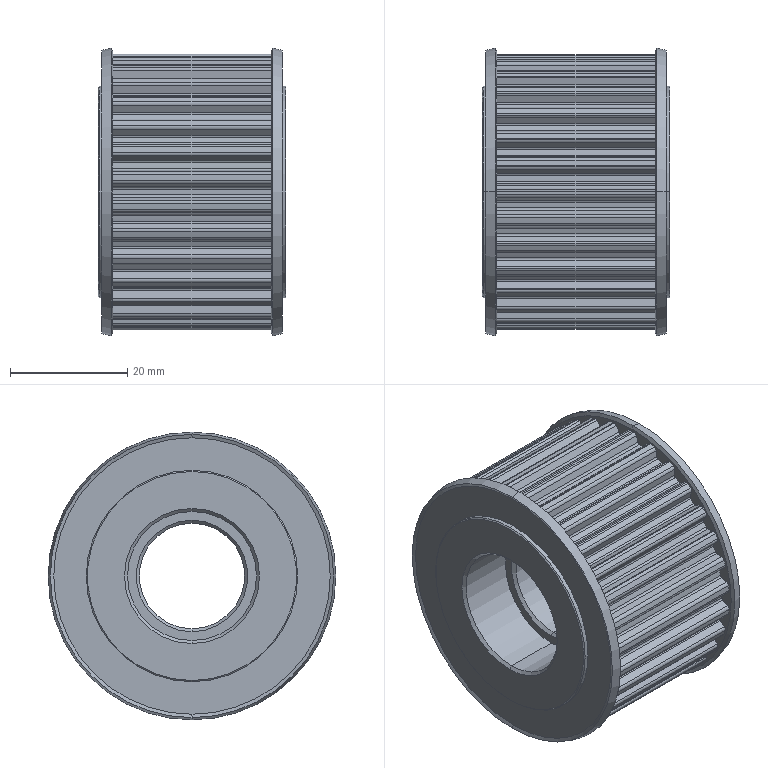Part | STEP file | PN_0019 T5 synchronous pulley 30 teeth 2 | 1 solid | 301 faces | box 32 x 49 x 49 mm | volume 40684 mm3 | cylinder 211 | plane 68 | cone 22 | commonest cylinder face diameters 0.8 x70 1.2 x70 46.95 x31 43.35 x30 22 x4 36 x4